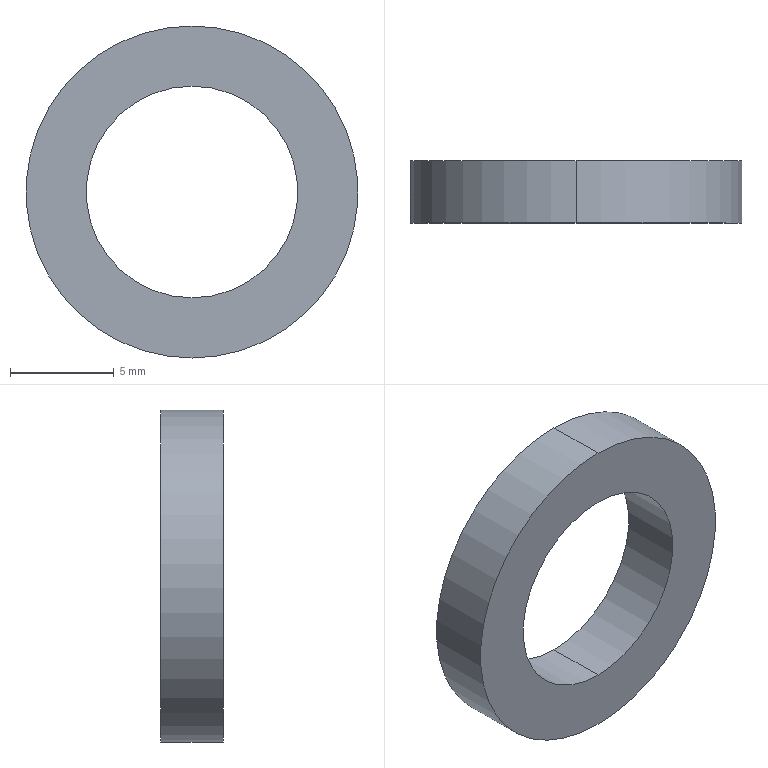Part | STEP file | BCC3 H12_12 | 1 solid | 6 faces | box 16 x 3 x 16 mm | volume 358.047 mm3 | cylinder 4 | plane 2 | commonest cylinder face diameters 10.2 x2 16 x2
STEP:
#1=CARTESIAN_POINT('',(0.,0.,0.));
#2=DIRECTION('',(0.,0.,1.));
#3=DIRECTION('',(1.,0.,0.));
#4=AXIS2_PLACEMENT_3D('',#1,#2,#3);
#5=CARTESIAN_POINT('',(0.,3.,-5.1));
#6=VERTEX_POINT('',#5);
#7=CARTESIAN_POINT('',(0.,0.,-5.1));
#8=VERTEX_POINT('',#7);
#9=CARTESIAN_POINT('',(0.,3.,-5.1));
#10=DIRECTION('',(0.,-1.,0.));
#11=VECTOR('',#10,1.);
#12=LINE('',#9,#11);
#13=CARTESIAN_POINT('',(0.,3.,0.));
#14=DIRECTION('',(0.,-1.,0.));
#15=DIRECTION('',(0.,0.,-1.));
#16=AXIS2_PLACEMENT_3D('',#13,#14,#15);
#17=CYLINDRICAL_SURFACE('',#16,5.1);
#18=CARTESIAN_POINT('',(6.283,0.));
#19=DIRECTION('',(0.,1.));
#20=VECTOR('',#19,1.);
#21=LINE('',#18,#20);
#22=(GEOMETRIC_REPRESENTATION_CONTEXT(2)PARAMETRIC_REPRESENTATION_CONTEXT()REPRESENTATION_CONTEXT('',''));
#23=DEFINITIONAL_REPRESENTATION('',(#21),#22);
#24=PCURVE('',#17,#23);
#25=CARTESIAN_POINT('',(0.,3.,0.));
#26=DIRECTION('',(0.,-1.,0.));
#27=DIRECTION('',(0.,0.,-1.));
#28=AXIS2_PLACEMENT_3D('',#25,#26,#27);
#29=CYLINDRICAL_SURFACE('',#28,5.1);
#30=CARTESIAN_POINT('',(0.,0.));
#31=DIRECTION('',(0.,1.));
#32=VECTOR('',#31,1.);
#33=LINE('',#30,#32);
#34=(GEOMETRIC_REPRESENTATION_CONTEXT(2)PARAMETRIC_REPRESENTATION_CONTEXT()REPRESENTATION_CONTEXT('',''));
#35=DEFINITIONAL_REPRESENTATION('',(#33),#34);
#36=PCURVE('',#29,#35);
#37=SURFACE_CURVE('',#12,(#24,#36),.PCURVE_S1.);
#38=EDGE_CURVE('',#6,#8,#37,.T.);
#39=ORIENTED_EDGE('',*,*,#38,.T.);
#40=CARTESIAN_POINT('',(0.,0.,5.1));
#41=VERTEX_POINT('',#40);
#42=CARTESIAN_POINT('',(0.,0.,0.));
#43=DIRECTION('',(0.,1.,0.));
#44=DIRECTION('',(0.,0.,1.));
#45=AXIS2_PLACEMENT_3D('',#42,#43,#44);
#46=CIRCLE('',#45,5.1);
#47=CARTESIAN_POINT('',(9.425,3.));
#48=DIRECTION('',(-1.,0.));
#49=VECTOR('',#48,1.);
#50=LINE('',#47,#49);
#51=(GEOMETRIC_REPRESENTATION_CONTEXT(2)PARAMETRIC_REPRESENTATION_CONTEXT()REPRESENTATION_CONTEXT('',''));
#52=DEFINITIONAL_REPRESENTATION('',(#50),#51);
#53=PCURVE('',#17,#52);
#54=CARTESIAN_POINT('',(0.,0.,0.));
#55=DIRECTION('',(0.,1.,0.));
#56=DIRECTION('',(0.,0.,1.));
#57=AXIS2_PLACEMENT_3D('',#54,#55,#56);
#58=PLANE('',#57);
#59=CARTESIAN_POINT('',(0.,0.));
#60=DIRECTION('',(1.,0.));
#61=AXIS2_PLACEMENT_2D('',#59,#60);
#62=CIRCLE('',#61,5.1);
#63=(GEOMETRIC_REPRESENTATION_CONTEXT(2)PARAMETRIC_REPRESENTATION_CONTEXT()REPRESENTATION_CONTEXT('',''));
#64=DEFINITIONAL_REPRESENTATION('',(#62),#63);
#65=PCURVE('',#58,#64);
#66=SURFACE_CURVE('',#46,(#53,#65),.PCURVE_S1.);
#67=EDGE_CURVE('',#8,#41,#66,.T.);
#68=ORIENTED_EDGE('',*,*,#67,.T.);
#69=CARTESIAN_POINT('',(0.,3.,5.1));
#70=VERTEX_POINT('',#69);
#71=CARTESIAN_POINT('',(0.,3.,5.1));
#72=DIRECTION('',(0.,-1.,0.));
#73=VECTOR('',#72,1.);
#74=LINE('',#71,#73);
#75=CARTESIAN_POINT('',(3.142,0.));
#76=DIRECTION('',(0.,1.));
#77=VECTOR('',#76,1.);
#78=LINE('',#75,#77);
#79=(GEOMETRIC_REPRESENTATION_CONTEXT(2)PARAMETRIC_REPRESENTATION_CONTEXT()REPRESENTATION_CONTEXT('',''));
#80=DEFINITIONAL_REPRESENTATION('',(#78),#79);
#81=PCURVE('',#17,#80);
#82=CARTESIAN_POINT('',(3.142,0.));
#83=DIRECTION('',(0.,1.));
#84=VECTOR('',#83,1.);
#85=LINE('',#82,#84);
#86=(GEOMETRIC_REPRESENTATION_CONTEXT(2)PARAMETRIC_REPRESENTATION_CONTEXT()REPRESENTATION_CONTEXT('',''));
#87=DEFINITIONAL_REPRESENTATION('',(#85),#86);
#88=PCURVE('',#29,#87);
#89=SURFACE_CURVE('',#74,(#81,#88),.PCURVE_S1.);
#90=EDGE_CURVE('',#70,#41,#89,.T.);
#91=ORIENTED_EDGE('',*,*,#90,.F.);
#92=CARTESIAN_POINT('',(0.,3.,0.));
#93=DIRECTION('',(0.,1.,0.));
#94=DIRECTION('',(0.,0.,1.));
#95=AXIS2_PLACEMENT_3D('',#92,#93,#94);
#96=CIRCLE('',#95,5.1);
#97=CARTESIAN_POINT('',(9.425,0.));
#98=DIRECTION('',(-1.,0.));
#99=VECTOR('',#98,1.);
#100=LINE('',#97,#99);
#101=(GEOMETRIC_REPRESENTATION_CONTEXT(2)PARAMETRIC_REPRESENTATION_CONTEXT()REPRESENTATION_CONTEXT('',''));
#102=DEFINITIONAL_REPRESENTATION('',(#100),#101);
#103=PCURVE('',#17,#102);
#104=CARTESIAN_POINT('',(0.,3.,0.));
#105=DIRECTION('',(0.,1.,0.));
#106=DIRECTION('',(0.,0.,1.));
#107=AXIS2_PLACEMENT_3D('',#104,#105,#106);
#108=PLANE('',#107);
#109=CARTESIAN_POINT('',(0.,0.));
#110=DIRECTION('',(1.,0.));
#111=AXIS2_PLACEMENT_2D('',#109,#110);
#112=CIRCLE('',#111,5.1);
#113=(GEOMETRIC_REPRESENTATION_CONTEXT(2)PARAMETRIC_REPRESENTATION_CONTEXT()REPRESENTATION_CONTEXT('',''));
#114=DEFINITIONAL_REPRESENTATION('',(#112),#113);
#115=PCURVE('',#108,#114);
#116=SURFACE_CURVE('',#96,(#103,#115),.PCURVE_S1.);
#117=EDGE_CURVE('',#6,#70,#116,.T.);
#118=ORIENTED_EDGE('',*,*,#117,.F.);
#119=EDGE_LOOP('',(#39,#68,#91,#118));
#120=FACE_BOUND('',#119,.F.);
#121=ADVANCED_FACE('',(#120),#17,.F.);
#122=CARTESIAN_POINT('',(0.,3.,8.));
#123=VERTEX_POINT('',#122);
#124=CARTESIAN_POINT('',(0.,3.,-8.));
#125=VERTEX_POINT('',#124);
#126=CARTESIAN_POINT('',(0.,3.,0.));
#127=DIRECTION('',(0.,1.,0.));
#128=DIRECTION('',(0.,0.,1.));
#129=AXIS2_PLACEMENT_3D('',#126,#127,#128);
#130=CIRCLE('',#129,8.);
#131=CARTESIAN_POINT('',(0.,3.,0.));
#132=DIRECTION('',(0.,-1.,0.));
#133=DIRECTION('',(0.,0.,-1.));
#134=AXIS2_PLACEMENT_3D('',#131,#132,#133);
#135=CYLINDRICAL_SURFACE('',#134,8.);
#136=CARTESIAN_POINT('',(3.142,0.));
#137=DIRECTION('',(-1.,0.));
#138=VECTOR('',#137,1.);
#139=LINE('',#136,#138);
#140=(GEOMETRIC_REPRESENTATION_CONTEXT(2)PARAMETRIC_REPRESENTATION_CONTEXT()REPRESENTATION_CONTEXT('',''));
#141=DEFINITIONAL_REPRESENTATION('',(#139),#140);
#142=PCURVE('',#135,#141);
#143=CARTESIAN_POINT('',(0.,0.));
#144=DIRECTION('',(1.,0.));
#145=AXIS2_PLACEMENT_2D('',#143,#144);
#146=CIRCLE('',#145,8.);
#147=(GEOMETRIC_REPRESENTATION_CONTEXT(2)PARAMETRIC_REPRESENTATION_CONTEXT()REPRESENTATION_CONTEXT('',''));
#148=DEFINITIONAL_REPRESENTATION('',(#146),#147);
#149=PCURVE('',#108,#148);
#150=SURFACE_CURVE('',#130,(#142,#149),.PCURVE_S1.);
#151=EDGE_CURVE('',#123,#125,#150,.T.);
#152=ORIENTED_EDGE('',*,*,#151,.F.);
#153=CARTESIAN_POINT('',(0.,0.,8.));
#154=VERTEX_POINT('',#153);
#155=CARTESIAN_POINT('',(0.,3.,8.));
#156=DIRECTION('',(0.,-1.,0.));
#157=VECTOR('',#156,1.);
#158=LINE('',#155,#157);
#159=CARTESIAN_POINT('',(3.142,0.));
#160=DIRECTION('',(0.,1.));
#161=VECTOR('',#160,1.);
#162=LINE('',#159,#161);
#163=(GEOMETRIC_REPRESENTATION_CONTEXT(2)PARAMETRIC_REPRESENTATION_CONTEXT()REPRESENTATION_CONTEXT('',''));
#164=DEFINITIONAL_REPRESENTATION('',(#162),#163);
#165=PCURVE('',#135,#164);
#166=CARTESIAN_POINT('',(0.,3.,0.));
#167=DIRECTION('',(0.,-1.,0.));
#168=DIRECTION('',(0.,0.,-1.));
#169=AXIS2_PLACEMENT_3D('',#166,#167,#168);
#170=CYLINDRICAL_SURFACE('',#169,8.);
#171=CARTESIAN_POINT('',(3.142,0.));
#172=DIRECTION('',(0.,1.));
#173=VECTOR('',#172,1.);
#174=LINE('',#171,#173);
#175=(GEOMETRIC_REPRESENTATION_CONTEXT(2)PARAMETRIC_REPRESENTATION_CONTEXT()REPRESENTATION_CONTEXT('',''));
#176=DEFINITIONAL_REPRESENTATION('',(#174),#175);
#177=PCURVE('',#170,#176);
#178=SURFACE_CURVE('',#158,(#165,#177),.PCURVE_S1.);
#179=EDGE_CURVE('',#123,#154,#178,.T.);
#180=ORIENTED_EDGE('',*,*,#179,.T.);
#181=CARTESIAN_POINT('',(0.,0.,-8.));
#182=VERTEX_POINT('',#181);
#183=CARTESIAN_POINT('',(0.,0.,0.));
#184=DIRECTION('',(0.,1.,0.));
#185=DIRECTION('',(0.,0.,1.));
#186=AXIS2_PLACEMENT_3D('',#183,#184,#185);
#187=CIRCLE('',#186,8.);
#188=CARTESIAN_POINT('',(3.142,3.));
#189=DIRECTION('',(-1.,0.));
#190=VECTOR('',#189,1.);
#191=LINE('',#188,#190);
#192=(GEOMETRIC_REPRESENTATION_CONTEXT(2)PARAMETRIC_REPRESENTATION_CONTEXT()REPRESENTATION_CONTEXT('',''));
#193=DEFINITIONAL_REPRESENTATION('',(#191),#192);
#194=PCURVE('',#135,#193);
#195=CARTESIAN_POINT('',(0.,0.));
#196=DIRECTION('',(1.,0.));
#197=AXIS2_PLACEMENT_2D('',#195,#196);
#198=CIRCLE('',#197,8.);
#199=(GEOMETRIC_REPRESENTATION_CONTEXT(2)PARAMETRIC_REPRESENTATION_CONTEXT()REPRESENTATION_CONTEXT('',''));
#200=DEFINITIONAL_REPRESENTATION('',(#198),#199);
#201=PCURVE('',#58,#200);
#202=SURFACE_CURVE('',#187,(#194,#201),.PCURVE_S1.);
#203=EDGE_CURVE('',#154,#182,#202,.T.);
#204=ORIENTED_EDGE('',*,*,#203,.T.);
#205=CARTESIAN_POINT('',(0.,3.,-8.));
#206=DIRECTION('',(0.,-1.,0.));
#207=VECTOR('',#206,1.);
#208=LINE('',#205,#207);
#209=CARTESIAN_POINT('',(0.,0.));
#210=DIRECTION('',(0.,1.));
#211=VECTOR('',#210,1.);
#212=LINE('',#209,#211);
#213=(GEOMETRIC_REPRESENTATION_CONTEXT(2)PARAMETRIC_REPRESENTATION_CONTEXT()REPRESENTATION_CONTEXT('',''));
#214=DEFINITIONAL_REPRESENTATION('',(#212),#213);
#215=PCURVE('',#135,#214);
#216=CARTESIAN_POINT('',(6.283,0.));
#217=DIRECTION('',(0.,1.));
#218=VECTOR('',#217,1.);
#219=LINE('',#216,#218);
#220=(GEOMETRIC_REPRESENTATION_CONTEXT(2)PARAMETRIC_REPRESENTATION_CONTEXT()REPRESENTATION_CONTEXT('',''));
#221=DEFINITIONAL_REPRESENTATION('',(#219),#220);
#222=PCURVE('',#170,#221);
#223=SURFACE_CURVE('',#208,(#215,#222),.PCURVE_S1.);
#224=EDGE_CURVE('',#125,#182,#223,.T.);
#225=ORIENTED_EDGE('',*,*,#224,.F.);
#226=EDGE_LOOP('',(#152,#180,#204,#225));
#227=FACE_BOUND('',#226,.T.);
#228=ADVANCED_FACE('',(#227),#135,.T.);
#229=CARTESIAN_POINT('',(0.,3.,0.));
#230=DIRECTION('',(0.,1.,0.));
#231=DIRECTION('',(0.,0.,1.));
#232=AXIS2_PLACEMENT_3D('',#229,#230,#231);
#233=CIRCLE('',#232,8.);
#234=CARTESIAN_POINT('',(0.,0.));
#235=DIRECTION('',(1.,0.));
#236=AXIS2_PLACEMENT_2D('',#234,#235);
#237=CIRCLE('',#236,8.);
#238=(GEOMETRIC_REPRESENTATION_CONTEXT(2)PARAMETRIC_REPRESENTATION_CONTEXT()REPRESENTATION_CONTEXT('',''));
#239=DEFINITIONAL_REPRESENTATION('',(#237),#238);
#240=PCURVE('',#108,#239);
#241=CARTESIAN_POINT('',(9.425,0.));
#242=DIRECTION('',(-1.,0.));
#243=VECTOR('',#242,1.);
#244=LINE('',#241,#243);
#245=(GEOMETRIC_REPRESENTATION_CONTEXT(2)PARAMETRIC_REPRESENTATION_CONTEXT()REPRESENTATION_CONTEXT('',''));
#246=DEFINITIONAL_REPRESENTATION('',(#244),#245);
#247=PCURVE('',#170,#246);
#248=SURFACE_CURVE('',#233,(#240,#247),.PCURVE_S1.);
#249=EDGE_CURVE('',#125,#123,#248,.T.);
#250=ORIENTED_EDGE('',*,*,#249,.T.);
#251=ORIENTED_EDGE('',*,*,#151,.T.);
#252=EDGE_LOOP('',(#250,#251));
#253=FACE_BOUND('',#252,.T.);
#254=ORIENTED_EDGE('',*,*,#117,.F.);
#255=CARTESIAN_POINT('',(0.,3.,0.));
#256=DIRECTION('',(0.,1.,0.));
#257=DIRECTION('',(0.,0.,1.));
#258=AXIS2_PLACEMENT_3D('',#255,#256,#257);
#259=CIRCLE('',#258,5.1);
#260=CARTESIAN_POINT('',(0.,0.));
#261=DIRECTION('',(1.,0.));
#262=AXIS2_PLACEMENT_2D('',#260,#261);
#263=CIRCLE('',#262,5.1);
#264=(GEOMETRIC_REPRESENTATION_CONTEXT(2)PARAMETRIC_REPRESENTATION_CONTEXT()REPRESENTATION_CONTEXT('',''));
#265=DEFINITIONAL_REPRESENTATION('',(#263),#264);
#266=PCURVE('',#108,#265);
#267=CARTESIAN_POINT('',(3.142,0.));
#268=DIRECTION('',(-1.,0.));
#269=VECTOR('',#268,1.);
#270=LINE('',#267,#269);
#271=(GEOMETRIC_REPRESENTATION_CONTEXT(2)PARAMETRIC_REPRESENTATION_CONTEXT()REPRESENTATION_CONTEXT('',''));
#272=DEFINITIONAL_REPRESENTATION('',(#270),#271);
#273=PCURVE('',#29,#272);
#274=SURFACE_CURVE('',#259,(#266,#273),.PCURVE_S1.);
#275=EDGE_CURVE('',#70,#6,#274,.T.);
#276=ORIENTED_EDGE('',*,*,#275,.F.);
#277=EDGE_LOOP('',(#254,#276));
#278=FACE_BOUND('',#277,.T.);
#279=ADVANCED_FACE('',(#253,#278),#108,.T.);
#280=CARTESIAN_POINT('',(0.,0.,0.));
#281=DIRECTION('',(0.,1.,0.));
#282=DIRECTION('',(0.,0.,1.));
#283=AXIS2_PLACEMENT_3D('',#280,#281,#282);
#284=CIRCLE('',#283,8.);
#285=CARTESIAN_POINT('',(0.,0.));
#286=DIRECTION('',(1.,0.));
#287=AXIS2_PLACEMENT_2D('',#285,#286);
#288=CIRCLE('',#287,8.);
#289=(GEOMETRIC_REPRESENTATION_CONTEXT(2)PARAMETRIC_REPRESENTATION_CONTEXT()REPRESENTATION_CONTEXT('',''));
#290=DEFINITIONAL_REPRESENTATION('',(#288),#289);
#291=PCURVE('',#58,#290);
#292=CARTESIAN_POINT('',(9.425,3.));
#293=DIRECTION('',(-1.,0.));
#294=VECTOR('',#293,1.);
#295=LINE('',#292,#294);
#296=(GEOMETRIC_REPRESENTATION_CONTEXT(2)PARAMETRIC_REPRESENTATION_CONTEXT()REPRESENTATION_CONTEXT('',''));
#297=DEFINITIONAL_REPRESENTATION('',(#295),#296);
#298=PCURVE('',#170,#297);
#299=SURFACE_CURVE('',#284,(#291,#298),.PCURVE_S1.);
#300=EDGE_CURVE('',#182,#154,#299,.T.);
#301=ORIENTED_EDGE('',*,*,#300,.F.);
#302=ORIENTED_EDGE('',*,*,#203,.F.);
#303=EDGE_LOOP('',(#301,#302));
#304=FACE_BOUND('',#303,.T.);
#305=ORIENTED_EDGE('',*,*,#67,.T.);
#306=CARTESIAN_POINT('',(0.,0.,0.));
#307=DIRECTION('',(0.,1.,0.));
#308=DIRECTION('',(0.,0.,1.));
#309=AXIS2_PLACEMENT_3D('',#306,#307,#308);
#310=CIRCLE('',#309,5.1);
#311=CARTESIAN_POINT('',(0.,0.));
#312=DIRECTION('',(1.,0.));
#313=AXIS2_PLACEMENT_2D('',#311,#312);
#314=CIRCLE('',#313,5.1);
#315=(GEOMETRIC_REPRESENTATION_CONTEXT(2)PARAMETRIC_REPRESENTATION_CONTEXT()REPRESENTATION_CONTEXT('',''));
#316=DEFINITIONAL_REPRESENTATION('',(#314),#315);
#317=PCURVE('',#58,#316);
#318=CARTESIAN_POINT('',(3.142,3.));
#319=DIRECTION('',(-1.,0.));
#320=VECTOR('',#319,1.);
#321=LINE('',#318,#320);
#322=(GEOMETRIC_REPRESENTATION_CONTEXT(2)PARAMETRIC_REPRESENTATION_CONTEXT()REPRESENTATION_CONTEXT('',''));
#323=DEFINITIONAL_REPRESENTATION('',(#321),#322);
#324=PCURVE('',#29,#323);
#325=SURFACE_CURVE('',#310,(#317,#324),.PCURVE_S1.);
#326=EDGE_CURVE('',#41,#8,#325,.T.);
#327=ORIENTED_EDGE('',*,*,#326,.T.);
#328=EDGE_LOOP('',(#305,#327));
#329=FACE_BOUND('',#328,.T.);
#330=ADVANCED_FACE('',(#304,#329),#58,.F.);
#331=ORIENTED_EDGE('',*,*,#179,.F.);
#332=ORIENTED_EDGE('',*,*,#249,.F.);
#333=ORIENTED_EDGE('',*,*,#224,.T.);
#334=ORIENTED_EDGE('',*,*,#300,.T.);
#335=EDGE_LOOP('',(#331,#332,#333,#334));
#336=FACE_BOUND('',#335,.T.);
#337=ADVANCED_FACE('',(#336),#170,.T.);
#338=ORIENTED_EDGE('',*,*,#326,.T.);
#339=ORIENTED_EDGE('',*,*,#38,.F.);
#340=ORIENTED_EDGE('',*,*,#275,.F.);
#341=ORIENTED_EDGE('',*,*,#90,.T.);
#342=EDGE_LOOP('',(#338,#339,#340,#341));
#343=FACE_BOUND('',#342,.F.);
#344=ADVANCED_FACE('',(#343),#29,.F.);
#345=CLOSED_SHELL('',(#121,#228,#279,#330,#337,#344));
#346=MANIFOLD_SOLID_BREP('',#345);
#347=(LENGTH_UNIT()NAMED_UNIT(*)SI_UNIT(.MILLI.,.METRE.));
#348=UNCERTAINTY_MEASURE_WITH_UNIT(LENGTH_MEASURE(0.0000001),#347,'','');
#349=(NAMED_UNIT(*)PLANE_ANGLE_UNIT()SI_UNIT($,.RADIAN.));
#350=(NAMED_UNIT(*)SI_UNIT($,.STERADIAN.)SOLID_ANGLE_UNIT());
#351=(GEOMETRIC_REPRESENTATION_CONTEXT(3)GLOBAL_UNCERTAINTY_ASSIGNED_CONTEXT((#348))GLOBAL_UNIT_ASSIGNED_CONTEXT((#347,#349,#350))REPRESENTATION_CONTEXT('',''));
#352=ADVANCED_BREP_SHAPE_REPRESENTATION('',(#4,#346),#351);